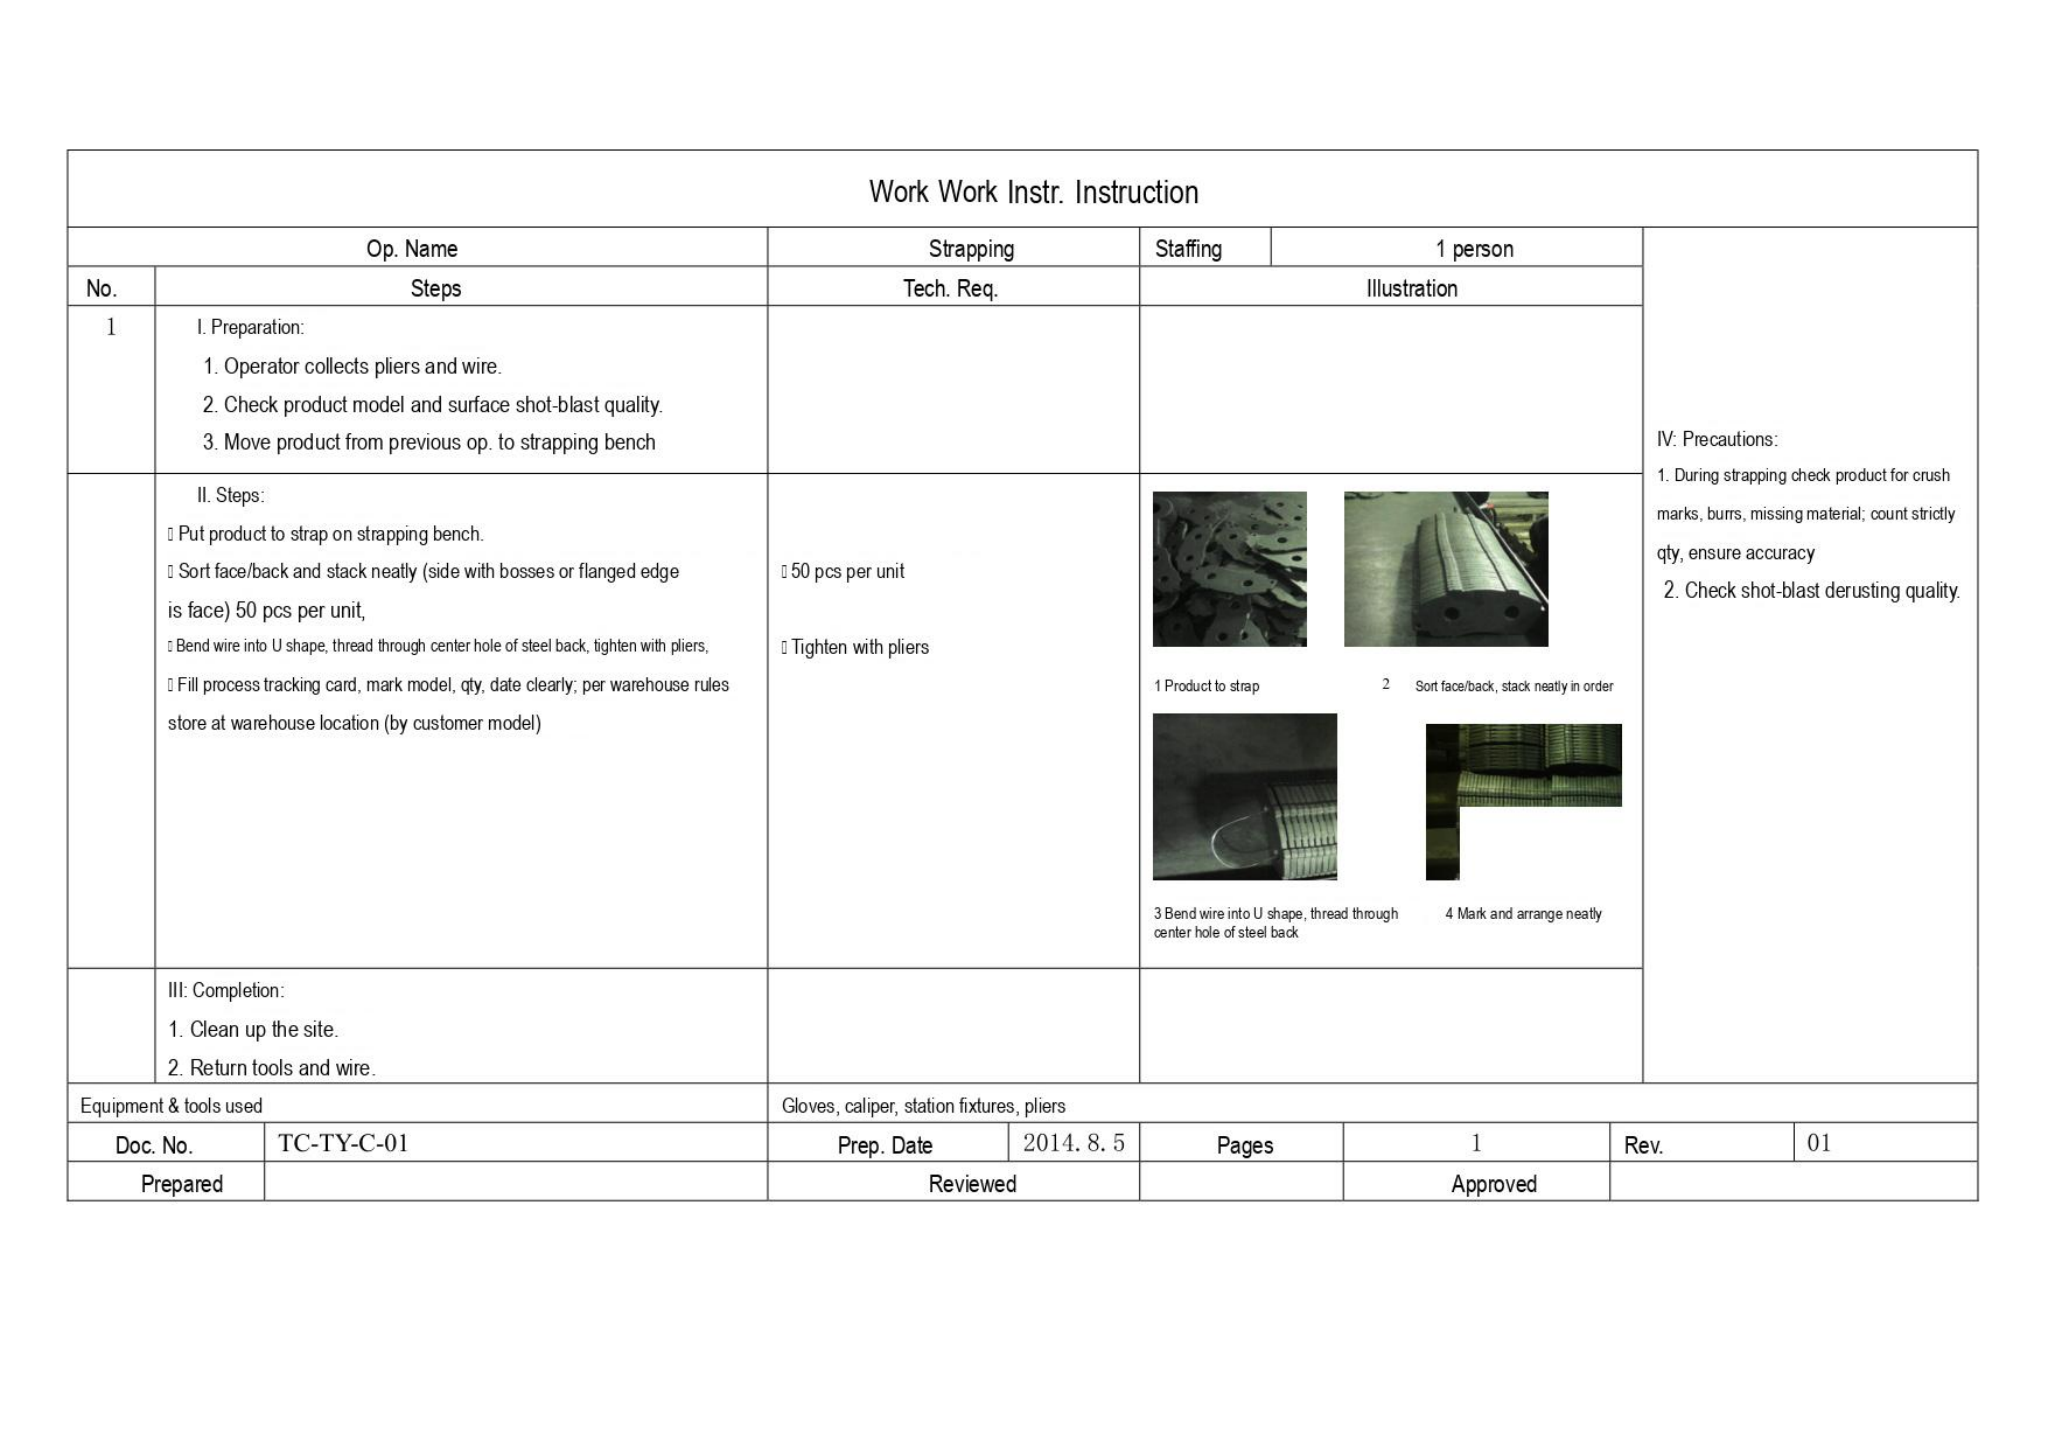# Work Work Instr. Instruction

| Op. Name | | Strapping | Staffing | 1 person |
|---|---|---|---|---|
| **No.** | **Steps** | **Tech. Req.** | **Illustration** | |
| 1 | I. Preparation:<br>1. Operator collects pliers and wire.<br>2. Check product model and surface shot-blast quality.<br>3. Move product from previous op. to strapping bench | | | IV: Precautions:<br>1. During strapping check product for crush marks, burrs, missing material; count strictly qty, ensure accuracy<br>2. Check shot-blast derusting quality. |
| | II. Steps:<br>▯ Put product to strap on strapping bench.<br>▯ Sort face/back and stack neatly (side with bosses or flanged edge is face) 50 pcs per unit,<br>▯ Bend wire into U shape, thread through center hole of steel back, tighten with pliers,<br>▯ Fill process tracking card, mark model, qty, date clearly; per warehouse rules store at warehouse location (by customer model) | ▯ 50 pcs per unit<br>▯ Tighten with pliers | 1 Product to strap<br>2 Sort face/back, stack neatly in order<br>3 Bend wire into U shape, thread through center hole of steel back<br>4 Mark and arrange neatly | |
| | III: Completion:<br>1. Clean up the site.<br>2. Return tools and wire. | | | |

| Equipment & tools used | Gloves, caliper, station fixtures, pliers | | | | | | |
|---|---|---|---|---|---|---|---|
| Doc. No. | TC-TY-C-01 | Prep. Date | 2014. 8. 5 | Pages | 1 | Rev. | 01 |
| Prepared | | Reviewed | | Approved | | | |